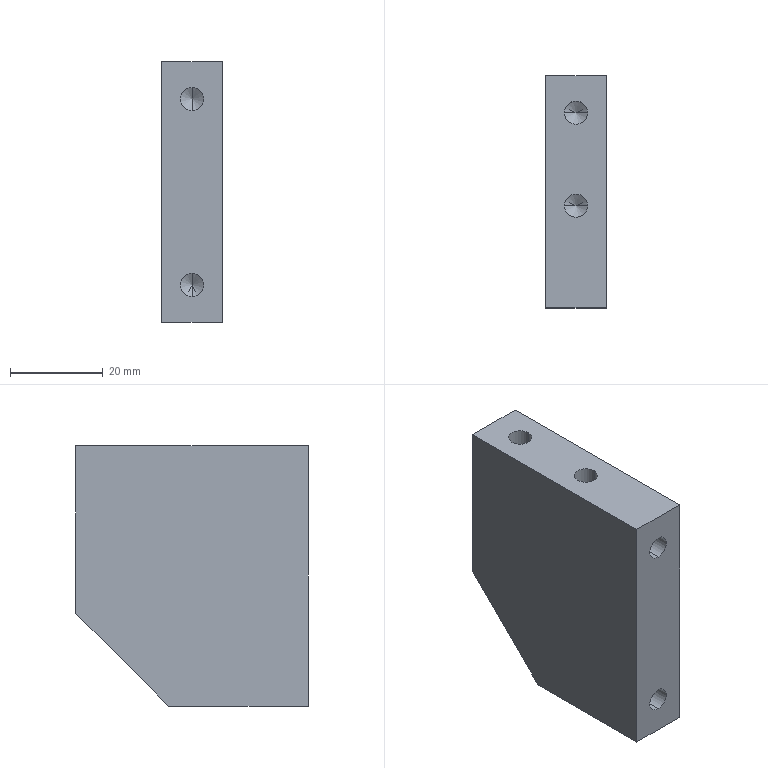Part | STEP file | OP10-122_rib plate | 1 solid | 23 faces | box 13 x 50 x 56 mm | volume 32347 mm3 | cylinder 8 | cone 8 | plane 7 | commonest cylinder face diameters 5 x8